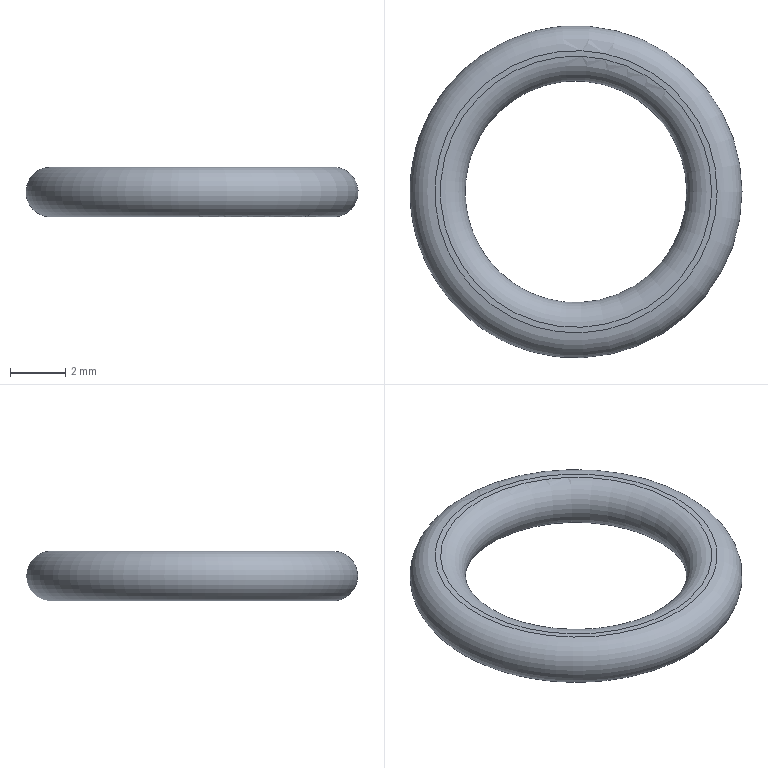Part | NX | features solid 2 | 1 solid | 4 faces | box 12 x 12 x 1.8 mm | volume 91.254 mm3 | plane 2 | torus 2
STEP:
#1=CARTESIAN_POINT('',(34.9,30.,-71.8));
#2=VERTEX_POINT('',#1);
#3=CARTESIAN_POINT('',(40.,30.,-71.8));
#4=DIRECTION('',(0.,0.,-1.));
#5=DIRECTION('',(-1.,0.,0.));
#6=AXIS2_PLACEMENT_3D('',#3,#4,#5);
#7=CIRCLE('',#6,5.1);
#8=EDGE_CURVE('',#2,#2,#7,.T.);
#9=ORIENTED_EDGE('',*,*,#8,.T.);
#10=EDGE_LOOP('',(#9));
#11=FACE_BOUND('',#10,.T.);
#12=CARTESIAN_POINT('',(35.1,30.,-71.8));
#13=VERTEX_POINT('',#12);
#14=CARTESIAN_POINT('',(40.,30.,-71.8));
#15=DIRECTION('',(0.,0.,-1.));
#16=DIRECTION('',(-1.,0.,0.));
#17=AXIS2_PLACEMENT_3D('',#14,#15,#16);
#18=CIRCLE('',#17,4.9);
#19=EDGE_CURVE('',#13,#13,#18,.F.);
#20=ORIENTED_EDGE('',*,*,#19,.T.);
#21=EDGE_LOOP('',(#20));
#22=FACE_BOUND('',#21,.T.);
#23=CARTESIAN_POINT('',(40.,30.,-71.8));
#24=DIRECTION('',(0.,0.,-1.));
#25=DIRECTION('',(-1.,0.,0.));
#26=AXIS2_PLACEMENT_3D('',#23,#24,#25);
#27=PLANE('',#26);
#28=ADVANCED_FACE('',(#11,#22),#27,.T.);
#29=CARTESIAN_POINT('',(45.1,30.,-70.));
#30=VERTEX_POINT('',#29);
#31=CARTESIAN_POINT('',(40.,30.,-70.));
#32=DIRECTION('',(0.,0.,1.));
#33=DIRECTION('',(1.,0.,0.));
#34=AXIS2_PLACEMENT_3D('',#31,#32,#33);
#35=CIRCLE('',#34,5.1);
#36=EDGE_CURVE('',#30,#30,#35,.T.);
#37=ORIENTED_EDGE('',*,*,#36,.T.);
#38=EDGE_LOOP('',(#37));
#39=FACE_BOUND('',#38,.T.);
#40=CARTESIAN_POINT('',(44.9,30.,-70.));
#41=VERTEX_POINT('',#40);
#42=CARTESIAN_POINT('',(40.,30.,-70.));
#43=DIRECTION('',(0.,0.,1.));
#44=DIRECTION('',(1.,0.,0.));
#45=AXIS2_PLACEMENT_3D('',#42,#43,#44);
#46=CIRCLE('',#45,4.9);
#47=EDGE_CURVE('',#41,#41,#46,.F.);
#48=ORIENTED_EDGE('',*,*,#47,.T.);
#49=EDGE_LOOP('',(#48));
#50=FACE_BOUND('',#49,.T.);
#51=CARTESIAN_POINT('',(40.,30.,-70.));
#52=DIRECTION('',(0.,0.,1.));
#53=DIRECTION('',(1.,0.,0.));
#54=AXIS2_PLACEMENT_3D('',#51,#52,#53);
#55=PLANE('',#54);
#56=ADVANCED_FACE('',(#39,#50),#55,.T.);
#57=ORIENTED_EDGE('',*,*,#36,.F.);
#58=EDGE_LOOP('',(#57));
#59=FACE_BOUND('',#58,.T.);
#60=ORIENTED_EDGE('',*,*,#8,.F.);
#61=EDGE_LOOP('',(#60));
#62=FACE_BOUND('',#61,.T.);
#63=CARTESIAN_POINT('',(40.,30.,-70.9));
#64=DIRECTION('',(0.,0.,1.));
#65=DIRECTION('',(1.,0.,0.));
#66=AXIS2_PLACEMENT_3D('',#63,#64,#65);
#67=TOROIDAL_SURFACE('',#66,5.1,0.9);
#68=ADVANCED_FACE('',(#59,#62),#67,.T.);
#69=ORIENTED_EDGE('',*,*,#47,.F.);
#70=EDGE_LOOP('',(#69));
#71=FACE_BOUND('',#70,.T.);
#72=ORIENTED_EDGE('',*,*,#19,.F.);
#73=EDGE_LOOP('',(#72));
#74=FACE_BOUND('',#73,.T.);
#75=CARTESIAN_POINT('',(40.,30.,-70.9));
#76=DIRECTION('',(0.,0.,1.));
#77=DIRECTION('',(1.,0.,0.));
#78=AXIS2_PLACEMENT_3D('',#75,#76,#77);
#79=TOROIDAL_SURFACE('',#78,4.9,0.9);
#80=ADVANCED_FACE('',(#71,#74),#79,.T.);
#81=CLOSED_SHELL('',(#28,#56,#68,#80));
#82=MANIFOLD_SOLID_BREP('',#81);
#83=(LENGTH_UNIT()NAMED_UNIT(*)SI_UNIT(.MILLI.,.METRE.));
#84=UNCERTAINTY_MEASURE_WITH_UNIT(LENGTH_MEASURE(0.00001),#83,'','');
#85=(NAMED_UNIT(*)PLANE_ANGLE_UNIT()SI_UNIT($,.RADIAN.));
#86=(NAMED_UNIT(*)SI_UNIT($,.STERADIAN.)SOLID_ANGLE_UNIT());
#87=(GEOMETRIC_REPRESENTATION_CONTEXT(3)GLOBAL_UNCERTAINTY_ASSIGNED_CONTEXT((#84))GLOBAL_UNIT_ASSIGNED_CONTEXT((#83,#85,#86))REPRESENTATION_CONTEXT('',''));
#88=ADVANCED_BREP_SHAPE_REPRESENTATION('',(#82),#87);